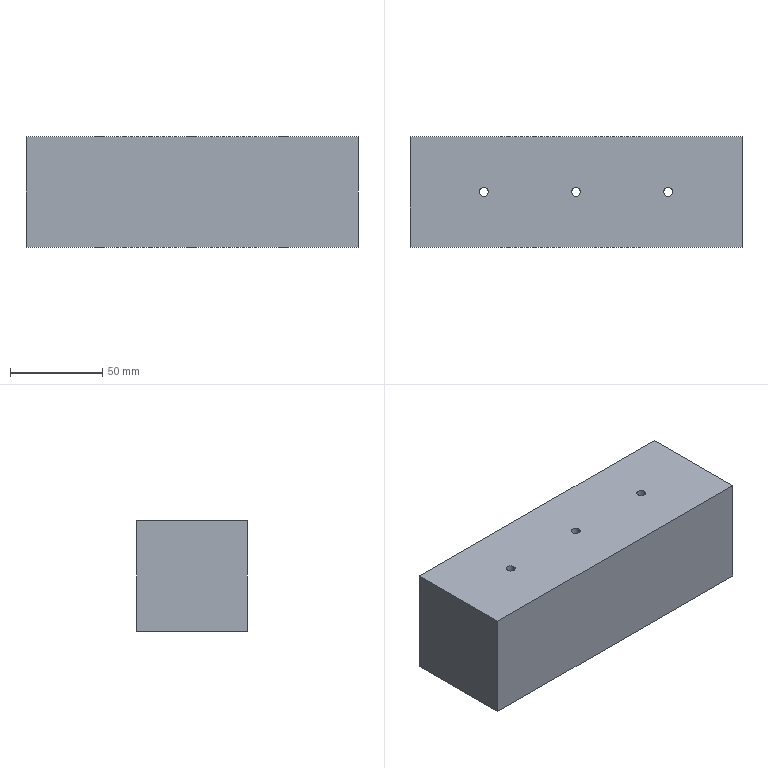Part | SolidWorks | features Extrusion 1, HoleWzd 1 | 1 solid | 12 faces | box 180 x 60 x 60 mm | volume 644743 mm3 | cylinder 6 | plane 6 | commonest cylinder face diameters 4.8 x6
STEP:
#1=CARTESIAN_POINT('',(2.4,30.,30.));
#2=VERTEX_POINT('',#1);
#3=CARTESIAN_POINT('',(-2.4,30.,30.));
#4=VERTEX_POINT('',#3);
#5=CARTESIAN_POINT('',(0.,30.,30.));
#6=DIRECTION('',(0.,0.,-1.));
#7=DIRECTION('',(-1.,0.,0.));
#8=AXIS2_PLACEMENT_3D('',#5,#6,#7);
#9=CIRCLE('',#8,2.4);
#10=EDGE_CURVE('',#2,#4,#9,.T.);
#11=ORIENTED_EDGE('',*,*,#10,.F.);
#12=CARTESIAN_POINT('',(2.4,30.,-30.));
#13=VERTEX_POINT('',#12);
#14=CARTESIAN_POINT('',(2.4,30.,-30.));
#15=DIRECTION('',(0.,0.,-1.));
#16=VECTOR('',#15,1000.);
#17=LINE('',#14,#16);
#18=EDGE_CURVE('',#2,#13,#17,.T.);
#19=ORIENTED_EDGE('',*,*,#18,.T.);
#20=CARTESIAN_POINT('',(-2.4,30.,-30.));
#21=VERTEX_POINT('',#20);
#22=CARTESIAN_POINT('',(0.,30.,-30.));
#23=DIRECTION('',(0.,0.,-1.));
#24=DIRECTION('',(-1.,0.,0.));
#25=AXIS2_PLACEMENT_3D('',#22,#23,#24);
#26=CIRCLE('',#25,2.4);
#27=EDGE_CURVE('',#13,#21,#26,.T.);
#28=ORIENTED_EDGE('',*,*,#27,.T.);
#29=CARTESIAN_POINT('',(-2.4,30.,-30.));
#30=DIRECTION('',(0.,0.,-1.));
#31=VECTOR('',#30,1000.);
#32=LINE('',#29,#31);
#33=EDGE_CURVE('',#4,#21,#32,.T.);
#34=ORIENTED_EDGE('',*,*,#33,.F.);
#35=EDGE_LOOP('',(#11,#19,#28,#34));
#36=FACE_OUTER_BOUND('',#35,.T.);
#37=CARTESIAN_POINT('',(0.,30.,-30.));
#38=DIRECTION('',(0.,0.,-1.));
#39=DIRECTION('',(-1.,0.,0.));
#40=AXIS2_PLACEMENT_3D('',#37,#38,#39);
#41=CYLINDRICAL_SURFACE('',#40,2.4);
#42=ADVANCED_FACE('',(#36),#41,.F.);
#43=CARTESIAN_POINT('',(-47.6,30.,30.));
#44=VERTEX_POINT('',#43);
#45=CARTESIAN_POINT('',(-52.4,30.,30.));
#46=VERTEX_POINT('',#45);
#47=CARTESIAN_POINT('',(-50.,30.,30.));
#48=DIRECTION('',(0.,0.,-1.));
#49=DIRECTION('',(-1.,0.,0.));
#50=AXIS2_PLACEMENT_3D('',#47,#48,#49);
#51=CIRCLE('',#50,2.4);
#52=EDGE_CURVE('',#44,#46,#51,.T.);
#53=ORIENTED_EDGE('',*,*,#52,.F.);
#54=CARTESIAN_POINT('',(-47.6,30.,-30.));
#55=VERTEX_POINT('',#54);
#56=CARTESIAN_POINT('',(-47.6,30.,-30.));
#57=DIRECTION('',(0.,0.,-1.));
#58=VECTOR('',#57,1000.);
#59=LINE('',#56,#58);
#60=EDGE_CURVE('',#44,#55,#59,.T.);
#61=ORIENTED_EDGE('',*,*,#60,.T.);
#62=CARTESIAN_POINT('',(-52.4,30.,-30.));
#63=VERTEX_POINT('',#62);
#64=CARTESIAN_POINT('',(-50.,30.,-30.));
#65=DIRECTION('',(0.,0.,-1.));
#66=DIRECTION('',(-1.,0.,0.));
#67=AXIS2_PLACEMENT_3D('',#64,#65,#66);
#68=CIRCLE('',#67,2.4);
#69=EDGE_CURVE('',#55,#63,#68,.T.);
#70=ORIENTED_EDGE('',*,*,#69,.T.);
#71=CARTESIAN_POINT('',(-52.4,30.,-30.));
#72=DIRECTION('',(0.,0.,-1.));
#73=VECTOR('',#72,1000.);
#74=LINE('',#71,#73);
#75=EDGE_CURVE('',#46,#63,#74,.T.);
#76=ORIENTED_EDGE('',*,*,#75,.F.);
#77=EDGE_LOOP('',(#53,#61,#70,#76));
#78=FACE_OUTER_BOUND('',#77,.T.);
#79=CARTESIAN_POINT('',(-50.,30.,-30.));
#80=DIRECTION('',(0.,0.,-1.));
#81=DIRECTION('',(-1.,0.,0.));
#82=AXIS2_PLACEMENT_3D('',#79,#80,#81);
#83=CYLINDRICAL_SURFACE('',#82,2.4);
#84=ADVANCED_FACE('',(#78),#83,.F.);
#85=CARTESIAN_POINT('',(52.4,30.,30.));
#86=VERTEX_POINT('',#85);
#87=CARTESIAN_POINT('',(47.6,30.,30.));
#88=VERTEX_POINT('',#87);
#89=CARTESIAN_POINT('',(50.,30.,30.));
#90=DIRECTION('',(0.,0.,-1.));
#91=DIRECTION('',(-1.,0.,0.));
#92=AXIS2_PLACEMENT_3D('',#89,#90,#91);
#93=CIRCLE('',#92,2.4);
#94=EDGE_CURVE('',#86,#88,#93,.T.);
#95=ORIENTED_EDGE('',*,*,#94,.F.);
#96=CARTESIAN_POINT('',(52.4,30.,-30.));
#97=VERTEX_POINT('',#96);
#98=CARTESIAN_POINT('',(52.4,30.,-30.));
#99=DIRECTION('',(0.,0.,-1.));
#100=VECTOR('',#99,1000.);
#101=LINE('',#98,#100);
#102=EDGE_CURVE('',#86,#97,#101,.T.);
#103=ORIENTED_EDGE('',*,*,#102,.T.);
#104=CARTESIAN_POINT('',(47.6,30.,-30.));
#105=VERTEX_POINT('',#104);
#106=CARTESIAN_POINT('',(50.,30.,-30.));
#107=DIRECTION('',(0.,0.,-1.));
#108=DIRECTION('',(-1.,0.,0.));
#109=AXIS2_PLACEMENT_3D('',#106,#107,#108);
#110=CIRCLE('',#109,2.4);
#111=EDGE_CURVE('',#97,#105,#110,.T.);
#112=ORIENTED_EDGE('',*,*,#111,.T.);
#113=CARTESIAN_POINT('',(47.6,30.,-30.));
#114=DIRECTION('',(0.,0.,-1.));
#115=VECTOR('',#114,1000.);
#116=LINE('',#113,#115);
#117=EDGE_CURVE('',#88,#105,#116,.T.);
#118=ORIENTED_EDGE('',*,*,#117,.F.);
#119=EDGE_LOOP('',(#95,#103,#112,#118));
#120=FACE_OUTER_BOUND('',#119,.T.);
#121=CARTESIAN_POINT('',(50.,30.,-30.));
#122=DIRECTION('',(0.,0.,-1.));
#123=DIRECTION('',(-1.,0.,0.));
#124=AXIS2_PLACEMENT_3D('',#121,#122,#123);
#125=CYLINDRICAL_SURFACE('',#124,2.4);
#126=ADVANCED_FACE('',(#120),#125,.F.);
#127=CARTESIAN_POINT('',(90.,0.,30.));
#128=VERTEX_POINT('',#127);
#129=CARTESIAN_POINT('',(90.,0.,-30.));
#130=VERTEX_POINT('',#129);
#131=CARTESIAN_POINT('',(90.,0.,30.));
#132=DIRECTION('',(0.,0.,-1.));
#133=VECTOR('',#132,1000.);
#134=LINE('',#131,#133);
#135=EDGE_CURVE('',#128,#130,#134,.T.);
#136=ORIENTED_EDGE('',*,*,#135,.T.);
#137=CARTESIAN_POINT('',(90.,60.,-30.));
#138=VERTEX_POINT('',#137);
#139=CARTESIAN_POINT('',(90.,60.,-30.));
#140=DIRECTION('',(0.,-1.,0.));
#141=VECTOR('',#140,1000.);
#142=LINE('',#139,#141);
#143=EDGE_CURVE('',#138,#130,#142,.T.);
#144=ORIENTED_EDGE('',*,*,#143,.F.);
#145=CARTESIAN_POINT('',(90.,60.,30.));
#146=VERTEX_POINT('',#145);
#147=CARTESIAN_POINT('',(90.,60.,30.));
#148=DIRECTION('',(0.,0.,-1.));
#149=VECTOR('',#148,1000.);
#150=LINE('',#147,#149);
#151=EDGE_CURVE('',#146,#138,#150,.T.);
#152=ORIENTED_EDGE('',*,*,#151,.F.);
#153=CARTESIAN_POINT('',(90.,60.,30.));
#154=DIRECTION('',(0.,-1.,0.));
#155=VECTOR('',#154,1000.);
#156=LINE('',#153,#155);
#157=EDGE_CURVE('',#146,#128,#156,.T.);
#158=ORIENTED_EDGE('',*,*,#157,.T.);
#159=EDGE_LOOP('',(#136,#144,#152,#158));
#160=FACE_OUTER_BOUND('',#159,.T.);
#161=CARTESIAN_POINT('',(90.,60.,30.));
#162=DIRECTION('',(-1.,0.,0.));
#163=DIRECTION('',(0.,0.,1.));
#164=AXIS2_PLACEMENT_3D('',#161,#162,#163);
#165=PLANE('',#164);
#166=ADVANCED_FACE('',(#160),#165,.F.);
#167=CARTESIAN_POINT('',(0.,30.,-30.));
#168=DIRECTION('',(0.,0.,-1.));
#169=DIRECTION('',(-1.,0.,0.));
#170=AXIS2_PLACEMENT_3D('',#167,#168,#169);
#171=CIRCLE('',#170,2.4);
#172=EDGE_CURVE('',#21,#13,#171,.T.);
#173=ORIENTED_EDGE('',*,*,#172,.F.);
#174=ORIENTED_EDGE('',*,*,#27,.F.);
#175=EDGE_LOOP('',(#173,#174));
#176=FACE_BOUND('',#175,.T.);
#177=CARTESIAN_POINT('',(-50.,30.,-30.));
#178=DIRECTION('',(0.,0.,-1.));
#179=DIRECTION('',(-1.,0.,0.));
#180=AXIS2_PLACEMENT_3D('',#177,#178,#179);
#181=CIRCLE('',#180,2.4);
#182=EDGE_CURVE('',#63,#55,#181,.T.);
#183=ORIENTED_EDGE('',*,*,#182,.F.);
#184=ORIENTED_EDGE('',*,*,#69,.F.);
#185=EDGE_LOOP('',(#183,#184));
#186=FACE_BOUND('',#185,.T.);
#187=CARTESIAN_POINT('',(50.,30.,-30.));
#188=DIRECTION('',(0.,0.,-1.));
#189=DIRECTION('',(-1.,0.,0.));
#190=AXIS2_PLACEMENT_3D('',#187,#188,#189);
#191=CIRCLE('',#190,2.4);
#192=EDGE_CURVE('',#105,#97,#191,.T.);
#193=ORIENTED_EDGE('',*,*,#192,.F.);
#194=ORIENTED_EDGE('',*,*,#111,.F.);
#195=EDGE_LOOP('',(#193,#194));
#196=FACE_BOUND('',#195,.T.);
#197=CARTESIAN_POINT('',(-90.,0.,-30.));
#198=VERTEX_POINT('',#197);
#199=CARTESIAN_POINT('',(-90.,0.,-30.));
#200=DIRECTION('',(-1.,0.,0.));
#201=VECTOR('',#200,1000.);
#202=LINE('',#199,#201);
#203=EDGE_CURVE('',#130,#198,#202,.T.);
#204=ORIENTED_EDGE('',*,*,#203,.T.);
#205=CARTESIAN_POINT('',(-90.,60.,-30.));
#206=VERTEX_POINT('',#205);
#207=CARTESIAN_POINT('',(-90.,60.,-30.));
#208=DIRECTION('',(0.,-1.,0.));
#209=VECTOR('',#208,1000.);
#210=LINE('',#207,#209);
#211=EDGE_CURVE('',#206,#198,#210,.T.);
#212=ORIENTED_EDGE('',*,*,#211,.F.);
#213=CARTESIAN_POINT('',(-90.,60.,-30.));
#214=DIRECTION('',(-1.,0.,0.));
#215=VECTOR('',#214,1000.);
#216=LINE('',#213,#215);
#217=EDGE_CURVE('',#138,#206,#216,.T.);
#218=ORIENTED_EDGE('',*,*,#217,.F.);
#219=ORIENTED_EDGE('',*,*,#143,.T.);
#220=EDGE_LOOP('',(#204,#212,#218,#219));
#221=FACE_OUTER_BOUND('',#220,.T.);
#222=CARTESIAN_POINT('',(-90.,60.,-30.));
#223=DIRECTION('',(0.,0.,1.));
#224=DIRECTION('',(1.,0.,0.));
#225=AXIS2_PLACEMENT_3D('',#222,#223,#224);
#226=PLANE('',#225);
#227=ADVANCED_FACE('',(#176,#186,#196,#221),#226,.F.);
#228=CARTESIAN_POINT('',(-90.,0.,30.));
#229=VERTEX_POINT('',#228);
#230=CARTESIAN_POINT('',(-90.,0.,30.));
#231=DIRECTION('',(0.,0.,1.));
#232=VECTOR('',#231,1000.);
#233=LINE('',#230,#232);
#234=EDGE_CURVE('',#198,#229,#233,.T.);
#235=ORIENTED_EDGE('',*,*,#234,.T.);
#236=CARTESIAN_POINT('',(-90.,60.,30.));
#237=VERTEX_POINT('',#236);
#238=CARTESIAN_POINT('',(-90.,60.,30.));
#239=DIRECTION('',(0.,-1.,0.));
#240=VECTOR('',#239,1000.);
#241=LINE('',#238,#240);
#242=EDGE_CURVE('',#237,#229,#241,.T.);
#243=ORIENTED_EDGE('',*,*,#242,.F.);
#244=CARTESIAN_POINT('',(-90.,60.,30.));
#245=DIRECTION('',(0.,0.,1.));
#246=VECTOR('',#245,1000.);
#247=LINE('',#244,#246);
#248=EDGE_CURVE('',#206,#237,#247,.T.);
#249=ORIENTED_EDGE('',*,*,#248,.F.);
#250=ORIENTED_EDGE('',*,*,#211,.T.);
#251=EDGE_LOOP('',(#235,#243,#249,#250));
#252=FACE_OUTER_BOUND('',#251,.T.);
#253=CARTESIAN_POINT('',(-90.,60.,30.));
#254=DIRECTION('',(1.,0.,0.));
#255=DIRECTION('',(0.,0.,-1.));
#256=AXIS2_PLACEMENT_3D('',#253,#254,#255);
#257=PLANE('',#256);
#258=ADVANCED_FACE('',(#252),#257,.F.);
#259=CARTESIAN_POINT('',(0.,30.,30.));
#260=DIRECTION('',(0.,0.,-1.));
#261=DIRECTION('',(-1.,0.,0.));
#262=AXIS2_PLACEMENT_3D('',#259,#260,#261);
#263=CIRCLE('',#262,2.4);
#264=EDGE_CURVE('',#4,#2,#263,.T.);
#265=ORIENTED_EDGE('',*,*,#264,.T.);
#266=ORIENTED_EDGE('',*,*,#10,.T.);
#267=EDGE_LOOP('',(#265,#266));
#268=FACE_BOUND('',#267,.T.);
#269=CARTESIAN_POINT('',(-50.,30.,30.));
#270=DIRECTION('',(0.,0.,-1.));
#271=DIRECTION('',(-1.,0.,0.));
#272=AXIS2_PLACEMENT_3D('',#269,#270,#271);
#273=CIRCLE('',#272,2.4);
#274=EDGE_CURVE('',#46,#44,#273,.T.);
#275=ORIENTED_EDGE('',*,*,#274,.T.);
#276=ORIENTED_EDGE('',*,*,#52,.T.);
#277=EDGE_LOOP('',(#275,#276));
#278=FACE_BOUND('',#277,.T.);
#279=CARTESIAN_POINT('',(50.,30.,30.));
#280=DIRECTION('',(0.,0.,-1.));
#281=DIRECTION('',(-1.,0.,0.));
#282=AXIS2_PLACEMENT_3D('',#279,#280,#281);
#283=CIRCLE('',#282,2.4);
#284=EDGE_CURVE('',#88,#86,#283,.T.);
#285=ORIENTED_EDGE('',*,*,#284,.T.);
#286=ORIENTED_EDGE('',*,*,#94,.T.);
#287=EDGE_LOOP('',(#285,#286));
#288=FACE_BOUND('',#287,.T.);
#289=CARTESIAN_POINT('',(-90.,0.,30.));
#290=DIRECTION('',(1.,0.,0.));
#291=VECTOR('',#290,1000.);
#292=LINE('',#289,#291);
#293=EDGE_CURVE('',#229,#128,#292,.T.);
#294=ORIENTED_EDGE('',*,*,#293,.T.);
#295=ORIENTED_EDGE('',*,*,#157,.F.);
#296=CARTESIAN_POINT('',(-90.,60.,30.));
#297=DIRECTION('',(1.,0.,0.));
#298=VECTOR('',#297,1000.);
#299=LINE('',#296,#298);
#300=EDGE_CURVE('',#237,#146,#299,.T.);
#301=ORIENTED_EDGE('',*,*,#300,.F.);
#302=ORIENTED_EDGE('',*,*,#242,.T.);
#303=EDGE_LOOP('',(#294,#295,#301,#302));
#304=FACE_OUTER_BOUND('',#303,.T.);
#305=CARTESIAN_POINT('',(-90.,60.,30.));
#306=DIRECTION('',(0.,0.,-1.));
#307=DIRECTION('',(-1.,0.,0.));
#308=AXIS2_PLACEMENT_3D('',#305,#306,#307);
#309=PLANE('',#308);
#310=ADVANCED_FACE('',(#268,#278,#288,#304),#309,.F.);
#311=ORIENTED_EDGE('',*,*,#151,.T.);
#312=ORIENTED_EDGE('',*,*,#217,.T.);
#313=ORIENTED_EDGE('',*,*,#248,.T.);
#314=ORIENTED_EDGE('',*,*,#300,.T.);
#315=EDGE_LOOP('',(#311,#312,#313,#314));
#316=FACE_OUTER_BOUND('',#315,.T.);
#317=CARTESIAN_POINT('',(0.,60.,0.));
#318=DIRECTION('',(0.,-1.,0.));
#319=DIRECTION('',(0.,0.,-1.));
#320=AXIS2_PLACEMENT_3D('',#317,#318,#319);
#321=PLANE('',#320);
#322=ADVANCED_FACE('',(#316),#321,.F.);
#323=ORIENTED_EDGE('',*,*,#135,.F.);
#324=ORIENTED_EDGE('',*,*,#293,.F.);
#325=ORIENTED_EDGE('',*,*,#234,.F.);
#326=ORIENTED_EDGE('',*,*,#203,.F.);
#327=EDGE_LOOP('',(#323,#324,#325,#326));
#328=FACE_OUTER_BOUND('',#327,.T.);
#329=CARTESIAN_POINT('',(0.,0.,0.));
#330=DIRECTION('',(0.,-1.,0.));
#331=DIRECTION('',(0.,0.,-1.));
#332=AXIS2_PLACEMENT_3D('',#329,#330,#331);
#333=PLANE('',#332);
#334=ADVANCED_FACE('',(#328),#333,.T.);
#335=ORIENTED_EDGE('',*,*,#102,.F.);
#336=ORIENTED_EDGE('',*,*,#284,.F.);
#337=ORIENTED_EDGE('',*,*,#117,.T.);
#338=ORIENTED_EDGE('',*,*,#192,.T.);
#339=EDGE_LOOP('',(#335,#336,#337,#338));
#340=FACE_OUTER_BOUND('',#339,.T.);
#341=CARTESIAN_POINT('',(50.,30.,-30.));
#342=DIRECTION('',(0.,0.,-1.));
#343=DIRECTION('',(-1.,0.,0.));
#344=AXIS2_PLACEMENT_3D('',#341,#342,#343);
#345=CYLINDRICAL_SURFACE('',#344,2.4);
#346=ADVANCED_FACE('',(#340),#345,.F.);
#347=ORIENTED_EDGE('',*,*,#60,.F.);
#348=ORIENTED_EDGE('',*,*,#274,.F.);
#349=ORIENTED_EDGE('',*,*,#75,.T.);
#350=ORIENTED_EDGE('',*,*,#182,.T.);
#351=EDGE_LOOP('',(#347,#348,#349,#350));
#352=FACE_OUTER_BOUND('',#351,.T.);
#353=CARTESIAN_POINT('',(-50.,30.,-30.));
#354=DIRECTION('',(0.,0.,-1.));
#355=DIRECTION('',(-1.,0.,0.));
#356=AXIS2_PLACEMENT_3D('',#353,#354,#355);
#357=CYLINDRICAL_SURFACE('',#356,2.4);
#358=ADVANCED_FACE('',(#352),#357,.F.);
#359=ORIENTED_EDGE('',*,*,#18,.F.);
#360=ORIENTED_EDGE('',*,*,#264,.F.);
#361=ORIENTED_EDGE('',*,*,#33,.T.);
#362=ORIENTED_EDGE('',*,*,#172,.T.);
#363=EDGE_LOOP('',(#359,#360,#361,#362));
#364=FACE_OUTER_BOUND('',#363,.T.);
#365=CARTESIAN_POINT('',(0.,30.,-30.));
#366=DIRECTION('',(0.,0.,-1.));
#367=DIRECTION('',(-1.,0.,0.));
#368=AXIS2_PLACEMENT_3D('',#365,#366,#367);
#369=CYLINDRICAL_SURFACE('',#368,2.4);
#370=ADVANCED_FACE('',(#364),#369,.F.);
#371=CLOSED_SHELL('',(#42,#84,#126,#166,#227,#258,#310,#322,#334,#346,#358,#370));
#372=MANIFOLD_SOLID_BREP('',#371);
#373=CARTESIAN_POINT('',(0.,0.,0.));
#374=DIRECTION('',(0.,0.,1.));
#375=DIRECTION('',(1.,0.,0.));
#376=AXIS2_PLACEMENT_3D('',#373,#374,#375);
#377=(LENGTH_UNIT()NAMED_UNIT(*)SI_UNIT(.MILLI.,.METRE.));
#378=UNCERTAINTY_MEASURE_WITH_UNIT(LENGTH_MEASURE(0.00001),#377,'','');
#379=(NAMED_UNIT(*)PLANE_ANGLE_UNIT()SI_UNIT($,.RADIAN.));
#380=(NAMED_UNIT(*)SI_UNIT($,.STERADIAN.)SOLID_ANGLE_UNIT());
#381=(GEOMETRIC_REPRESENTATION_CONTEXT(3)GLOBAL_UNCERTAINTY_ASSIGNED_CONTEXT((#378))GLOBAL_UNIT_ASSIGNED_CONTEXT((#377,#379,#380))REPRESENTATION_CONTEXT('',''));
#382=ADVANCED_BREP_SHAPE_REPRESENTATION('',(#372,#376),#381);